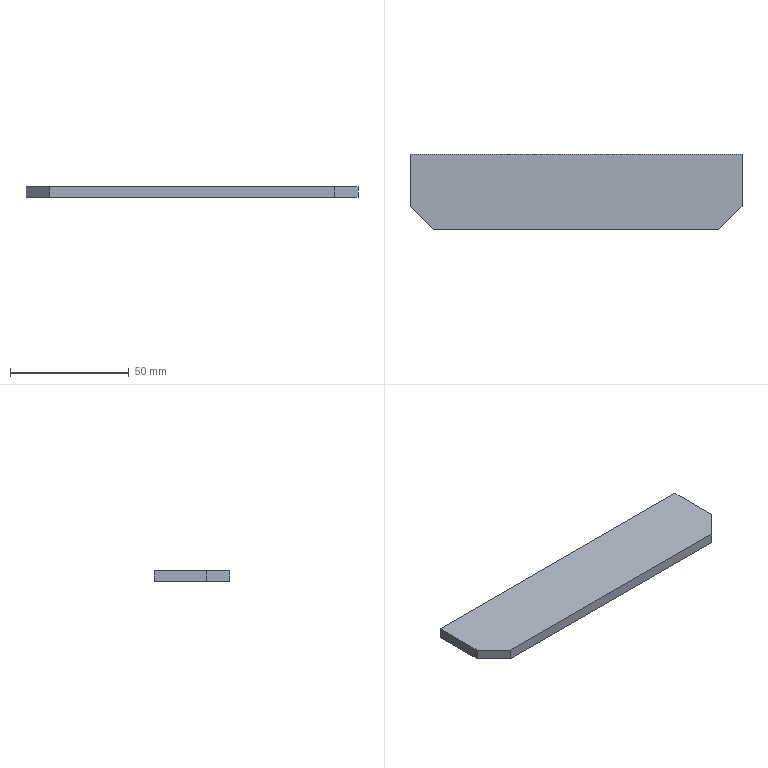Part | SolidWorks | features FlatPattern 1, SMBaseFlange 1, SheetMetal 1 | 1 solid | 8 faces | box 140 x 32 x 4.5 mm | volume 19710 mm3 | plane 8
STEP:
#1=CARTESIAN_POINT('',(-70.,16.,0.));
#2=VERTEX_POINT('',#1);
#3=CARTESIAN_POINT('',(-70.,-6.,0.));
#4=VERTEX_POINT('',#3);
#5=CARTESIAN_POINT('',(-70.,16.,0.));
#6=DIRECTION('',(0.,-1.,0.));
#7=VECTOR('',#6,1000.);
#8=LINE('',#5,#7);
#9=EDGE_CURVE('',#2,#4,#8,.T.);
#10=ORIENTED_EDGE('',*,*,#9,.F.);
#11=CARTESIAN_POINT('',(-70.,16.,-4.5));
#12=VERTEX_POINT('',#11);
#13=CARTESIAN_POINT('',(-70.,16.,-4.5));
#14=DIRECTION('',(0.,0.,1.));
#15=VECTOR('',#14,1000.);
#16=LINE('',#13,#15);
#17=EDGE_CURVE('',#12,#2,#16,.T.);
#18=ORIENTED_EDGE('',*,*,#17,.F.);
#19=CARTESIAN_POINT('',(-70.,-6.,-4.5));
#20=VERTEX_POINT('',#19);
#21=CARTESIAN_POINT('',(-70.,16.,-4.5));
#22=DIRECTION('',(0.,-1.,0.));
#23=VECTOR('',#22,1000.);
#24=LINE('',#21,#23);
#25=EDGE_CURVE('',#12,#20,#24,.T.);
#26=ORIENTED_EDGE('',*,*,#25,.T.);
#27=CARTESIAN_POINT('',(-70.,-6.,-4.5));
#28=DIRECTION('',(0.,0.,1.));
#29=VECTOR('',#28,1000.);
#30=LINE('',#27,#29);
#31=EDGE_CURVE('',#20,#4,#30,.T.);
#32=ORIENTED_EDGE('',*,*,#31,.T.);
#33=EDGE_LOOP('',(#10,#18,#26,#32));
#34=FACE_OUTER_BOUND('',#33,.T.);
#35=CARTESIAN_POINT('',(-70.,16.,-4.5));
#36=DIRECTION('',(-1.,0.,0.));
#37=DIRECTION('',(0.,0.,1.));
#38=AXIS2_PLACEMENT_3D('',#35,#36,#37);
#39=PLANE('',#38);
#40=ADVANCED_FACE('',(#34),#39,.T.);
#41=CARTESIAN_POINT('',(70.,16.,0.));
#42=VERTEX_POINT('',#41);
#43=CARTESIAN_POINT('',(-70.,16.,0.));
#44=DIRECTION('',(-1.,0.,0.));
#45=VECTOR('',#44,1000.);
#46=LINE('',#43,#45);
#47=EDGE_CURVE('',#42,#2,#46,.T.);
#48=ORIENTED_EDGE('',*,*,#47,.F.);
#49=CARTESIAN_POINT('',(70.,16.,-4.5));
#50=VERTEX_POINT('',#49);
#51=CARTESIAN_POINT('',(70.,16.,-4.5));
#52=DIRECTION('',(0.,0.,1.));
#53=VECTOR('',#52,1000.);
#54=LINE('',#51,#53);
#55=EDGE_CURVE('',#50,#42,#54,.T.);
#56=ORIENTED_EDGE('',*,*,#55,.F.);
#57=CARTESIAN_POINT('',(-70.,16.,-4.5));
#58=DIRECTION('',(-1.,0.,0.));
#59=VECTOR('',#58,1000.);
#60=LINE('',#57,#59);
#61=EDGE_CURVE('',#50,#12,#60,.T.);
#62=ORIENTED_EDGE('',*,*,#61,.T.);
#63=ORIENTED_EDGE('',*,*,#17,.T.);
#64=EDGE_LOOP('',(#48,#56,#62,#63));
#65=FACE_OUTER_BOUND('',#64,.T.);
#66=CARTESIAN_POINT('',(-70.,16.,-4.5));
#67=DIRECTION('',(0.,1.,0.));
#68=DIRECTION('',(0.,0.,1.));
#69=AXIS2_PLACEMENT_3D('',#66,#67,#68);
#70=PLANE('',#69);
#71=ADVANCED_FACE('',(#65),#70,.T.);
#72=CARTESIAN_POINT('',(70.,-6.,0.));
#73=VERTEX_POINT('',#72);
#74=CARTESIAN_POINT('',(70.,16.,0.));
#75=DIRECTION('',(0.,1.,0.));
#76=VECTOR('',#75,1000.);
#77=LINE('',#74,#76);
#78=EDGE_CURVE('',#73,#42,#77,.T.);
#79=ORIENTED_EDGE('',*,*,#78,.F.);
#80=CARTESIAN_POINT('',(70.,-6.,-4.5));
#81=VERTEX_POINT('',#80);
#82=CARTESIAN_POINT('',(70.,-6.,-4.5));
#83=DIRECTION('',(0.,0.,1.));
#84=VECTOR('',#83,1000.);
#85=LINE('',#82,#84);
#86=EDGE_CURVE('',#81,#73,#85,.T.);
#87=ORIENTED_EDGE('',*,*,#86,.F.);
#88=CARTESIAN_POINT('',(70.,16.,-4.5));
#89=DIRECTION('',(0.,1.,0.));
#90=VECTOR('',#89,1000.);
#91=LINE('',#88,#90);
#92=EDGE_CURVE('',#81,#50,#91,.T.);
#93=ORIENTED_EDGE('',*,*,#92,.T.);
#94=ORIENTED_EDGE('',*,*,#55,.T.);
#95=EDGE_LOOP('',(#79,#87,#93,#94));
#96=FACE_OUTER_BOUND('',#95,.T.);
#97=CARTESIAN_POINT('',(70.,16.,-4.5));
#98=DIRECTION('',(1.,0.,0.));
#99=DIRECTION('',(0.,1.,0.));
#100=AXIS2_PLACEMENT_3D('',#97,#98,#99);
#101=PLANE('',#100);
#102=ADVANCED_FACE('',(#96),#101,.T.);
#103=CARTESIAN_POINT('',(60.,-16.,0.));
#104=VERTEX_POINT('',#103);
#105=CARTESIAN_POINT('',(60.,-16.,0.));
#106=DIRECTION('',(0.7071,0.7071,0.));
#107=VECTOR('',#106,1000.);
#108=LINE('',#105,#107);
#109=EDGE_CURVE('',#104,#73,#108,.T.);
#110=ORIENTED_EDGE('',*,*,#109,.F.);
#111=CARTESIAN_POINT('',(60.,-16.,-4.5));
#112=VERTEX_POINT('',#111);
#113=CARTESIAN_POINT('',(60.,-16.,-4.5));
#114=DIRECTION('',(0.,0.,1.));
#115=VECTOR('',#114,1000.);
#116=LINE('',#113,#115);
#117=EDGE_CURVE('',#112,#104,#116,.T.);
#118=ORIENTED_EDGE('',*,*,#117,.F.);
#119=CARTESIAN_POINT('',(60.,-16.,-4.5));
#120=DIRECTION('',(0.7071,0.7071,0.));
#121=VECTOR('',#120,1000.);
#122=LINE('',#119,#121);
#123=EDGE_CURVE('',#112,#81,#122,.T.);
#124=ORIENTED_EDGE('',*,*,#123,.T.);
#125=ORIENTED_EDGE('',*,*,#86,.T.);
#126=EDGE_LOOP('',(#110,#118,#124,#125));
#127=FACE_OUTER_BOUND('',#126,.T.);
#128=CARTESIAN_POINT('',(60.,-16.,-4.5));
#129=DIRECTION('',(0.7071,-0.7071,0.));
#130=DIRECTION('',(0.7071,0.7071,0.));
#131=AXIS2_PLACEMENT_3D('',#128,#129,#130);
#132=PLANE('',#131);
#133=ADVANCED_FACE('',(#127),#132,.T.);
#134=CARTESIAN_POINT('',(-60.,-16.,0.));
#135=VERTEX_POINT('',#134);
#136=CARTESIAN_POINT('',(-60.,-16.,0.));
#137=DIRECTION('',(1.,0.,0.));
#138=VECTOR('',#137,1000.);
#139=LINE('',#136,#138);
#140=EDGE_CURVE('',#135,#104,#139,.T.);
#141=ORIENTED_EDGE('',*,*,#140,.F.);
#142=CARTESIAN_POINT('',(-60.,-16.,-4.5));
#143=VERTEX_POINT('',#142);
#144=CARTESIAN_POINT('',(-60.,-16.,-4.5));
#145=DIRECTION('',(0.,0.,1.));
#146=VECTOR('',#145,1000.);
#147=LINE('',#144,#146);
#148=EDGE_CURVE('',#143,#135,#147,.T.);
#149=ORIENTED_EDGE('',*,*,#148,.F.);
#150=CARTESIAN_POINT('',(-60.,-16.,-4.5));
#151=DIRECTION('',(1.,0.,0.));
#152=VECTOR('',#151,1000.);
#153=LINE('',#150,#152);
#154=EDGE_CURVE('',#143,#112,#153,.T.);
#155=ORIENTED_EDGE('',*,*,#154,.T.);
#156=ORIENTED_EDGE('',*,*,#117,.T.);
#157=EDGE_LOOP('',(#141,#149,#155,#156));
#158=FACE_OUTER_BOUND('',#157,.T.);
#159=CARTESIAN_POINT('',(-60.,-16.,-4.5));
#160=DIRECTION('',(0.,-1.,0.));
#161=DIRECTION('',(0.,0.,-1.));
#162=AXIS2_PLACEMENT_3D('',#159,#160,#161);
#163=PLANE('',#162);
#164=ADVANCED_FACE('',(#158),#163,.T.);
#165=CARTESIAN_POINT('',(-70.,-6.,0.));
#166=DIRECTION('',(0.7071,-0.7071,0.));
#167=VECTOR('',#166,1000.);
#168=LINE('',#165,#167);
#169=EDGE_CURVE('',#4,#135,#168,.T.);
#170=ORIENTED_EDGE('',*,*,#169,.F.);
#171=ORIENTED_EDGE('',*,*,#31,.F.);
#172=CARTESIAN_POINT('',(-70.,-6.,-4.5));
#173=DIRECTION('',(0.7071,-0.7071,0.));
#174=VECTOR('',#173,1000.);
#175=LINE('',#172,#174);
#176=EDGE_CURVE('',#20,#143,#175,.T.);
#177=ORIENTED_EDGE('',*,*,#176,.T.);
#178=ORIENTED_EDGE('',*,*,#148,.T.);
#179=EDGE_LOOP('',(#170,#171,#177,#178));
#180=FACE_OUTER_BOUND('',#179,.T.);
#181=CARTESIAN_POINT('',(-70.,-6.,-4.5));
#182=DIRECTION('',(-0.7071,-0.7071,0.));
#183=DIRECTION('',(0.7071,-0.7071,0.));
#184=AXIS2_PLACEMENT_3D('',#181,#182,#183);
#185=PLANE('',#184);
#186=ADVANCED_FACE('',(#180),#185,.T.);
#187=ORIENTED_EDGE('',*,*,#25,.F.);
#188=ORIENTED_EDGE('',*,*,#61,.F.);
#189=ORIENTED_EDGE('',*,*,#92,.F.);
#190=ORIENTED_EDGE('',*,*,#123,.F.);
#191=ORIENTED_EDGE('',*,*,#154,.F.);
#192=ORIENTED_EDGE('',*,*,#176,.F.);
#193=EDGE_LOOP('',(#187,#188,#189,#190,#191,#192));
#194=FACE_OUTER_BOUND('',#193,.T.);
#195=CARTESIAN_POINT('',(0.,0.,-4.5));
#196=DIRECTION('',(0.,0.,1.));
#197=DIRECTION('',(1.,0.,0.));
#198=AXIS2_PLACEMENT_3D('',#195,#196,#197);
#199=PLANE('',#198);
#200=ADVANCED_FACE('',(#194),#199,.F.);
#201=ORIENTED_EDGE('',*,*,#9,.T.);
#202=ORIENTED_EDGE('',*,*,#169,.T.);
#203=ORIENTED_EDGE('',*,*,#140,.T.);
#204=ORIENTED_EDGE('',*,*,#109,.T.);
#205=ORIENTED_EDGE('',*,*,#78,.T.);
#206=ORIENTED_EDGE('',*,*,#47,.T.);
#207=EDGE_LOOP('',(#201,#202,#203,#204,#205,#206));
#208=FACE_OUTER_BOUND('',#207,.T.);
#209=CARTESIAN_POINT('',(0.,0.,0.));
#210=DIRECTION('',(0.,0.,1.));
#211=DIRECTION('',(1.,0.,0.));
#212=AXIS2_PLACEMENT_3D('',#209,#210,#211);
#213=PLANE('',#212);
#214=ADVANCED_FACE('',(#208),#213,.T.);
#215=CLOSED_SHELL('',(#40,#71,#102,#133,#164,#186,#200,#214));
#216=MANIFOLD_SOLID_BREP('',#215);
#217=CARTESIAN_POINT('',(0.,0.,0.));
#218=DIRECTION('',(0.,0.,1.));
#219=DIRECTION('',(1.,0.,0.));
#220=AXIS2_PLACEMENT_3D('',#217,#218,#219);
#221=(LENGTH_UNIT()NAMED_UNIT(*)SI_UNIT(.MILLI.,.METRE.));
#222=UNCERTAINTY_MEASURE_WITH_UNIT(LENGTH_MEASURE(0.00001),#221,'','');
#223=(NAMED_UNIT(*)PLANE_ANGLE_UNIT()SI_UNIT($,.RADIAN.));
#224=(NAMED_UNIT(*)SI_UNIT($,.STERADIAN.)SOLID_ANGLE_UNIT());
#225=(GEOMETRIC_REPRESENTATION_CONTEXT(3)GLOBAL_UNCERTAINTY_ASSIGNED_CONTEXT((#222))GLOBAL_UNIT_ASSIGNED_CONTEXT((#221,#223,#224))REPRESENTATION_CONTEXT('',''));
#226=ADVANCED_BREP_SHAPE_REPRESENTATION('',(#216,#220),#225);